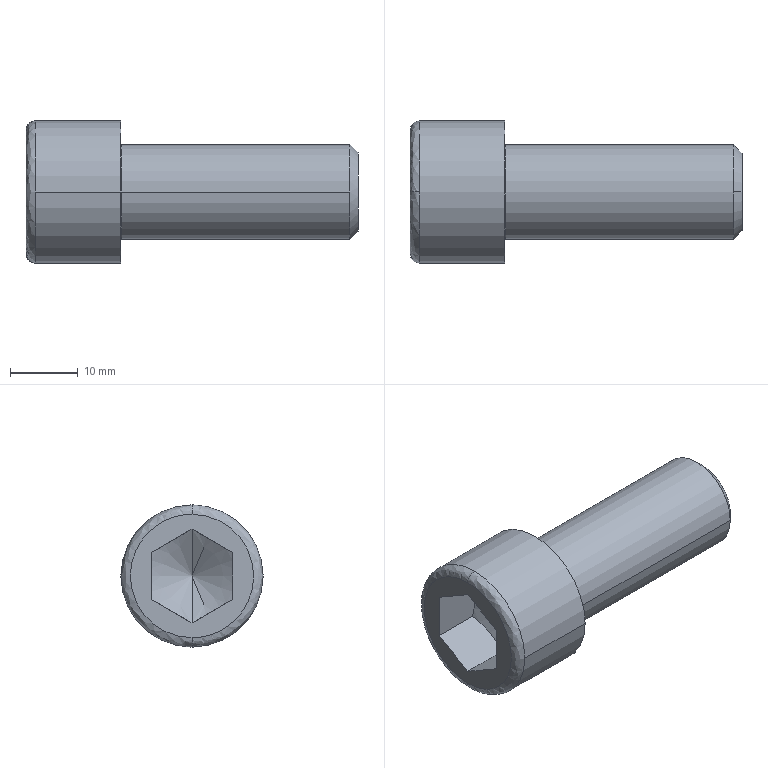Part | STEP file | DIN 912 - replaced by DIN EN ISO 4762 M14 x 35 | 1 solid | 21 faces | box 49 x 21 x 21 mm | volume 9111 mm3 | plane 9 | spline 4 | cylinder 4 | cone 4 | commonest cylinder face diameters 14 x2 21 x2